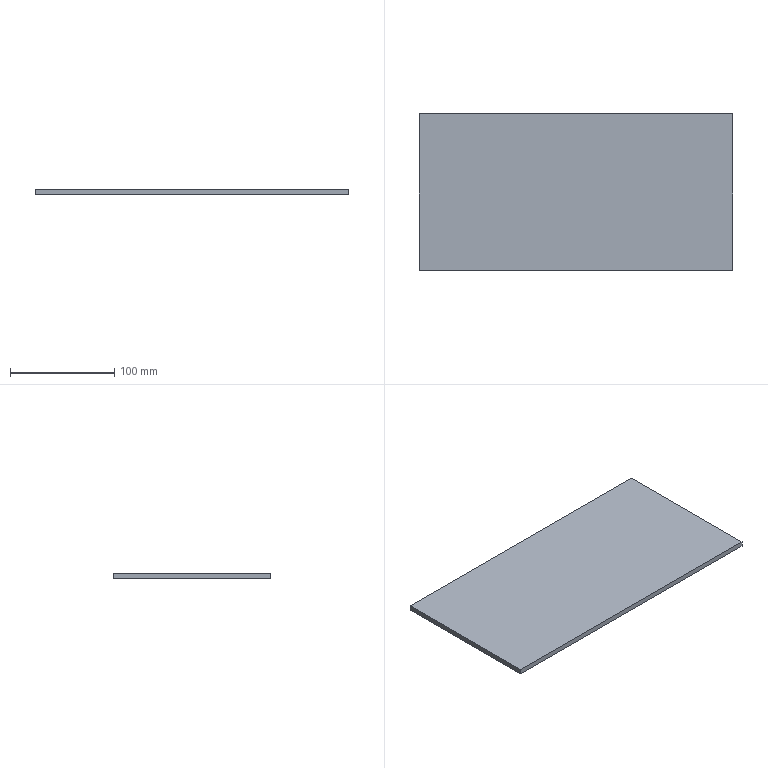Part | SolidWorks | features Extrusion 1 | 1 solid | 6 faces | box 300 x 150 x 5 mm | volume 225000 mm3 | plane 6
STEP:
#1=CARTESIAN_POINT('',(0.,150.,0.));
#2=VERTEX_POINT('',#1);
#3=CARTESIAN_POINT('',(0.,0.,0.));
#4=VERTEX_POINT('',#3);
#5=CARTESIAN_POINT('',(0.,0.,0.));
#6=DIRECTION('',(0.,-1.,0.));
#7=VECTOR('',#6,1000.);
#8=LINE('',#5,#7);
#9=EDGE_CURVE('',#2,#4,#8,.T.);
#10=ORIENTED_EDGE('',*,*,#9,.T.);
#11=CARTESIAN_POINT('',(0.,0.,5.));
#12=VERTEX_POINT('',#11);
#13=CARTESIAN_POINT('',(0.,0.,5.));
#14=DIRECTION('',(0.,0.,-1.));
#15=VECTOR('',#14,1000.);
#16=LINE('',#13,#15);
#17=EDGE_CURVE('',#12,#4,#16,.T.);
#18=ORIENTED_EDGE('',*,*,#17,.F.);
#19=CARTESIAN_POINT('',(0.,150.,5.));
#20=VERTEX_POINT('',#19);
#21=CARTESIAN_POINT('',(0.,0.,5.));
#22=DIRECTION('',(0.,-1.,0.));
#23=VECTOR('',#22,1000.);
#24=LINE('',#21,#23);
#25=EDGE_CURVE('',#20,#12,#24,.T.);
#26=ORIENTED_EDGE('',*,*,#25,.F.);
#27=CARTESIAN_POINT('',(0.,150.,5.));
#28=DIRECTION('',(0.,0.,-1.));
#29=VECTOR('',#28,1000.);
#30=LINE('',#27,#29);
#31=EDGE_CURVE('',#20,#2,#30,.T.);
#32=ORIENTED_EDGE('',*,*,#31,.T.);
#33=EDGE_LOOP('',(#10,#18,#26,#32));
#34=FACE_OUTER_BOUND('',#33,.T.);
#35=CARTESIAN_POINT('',(0.,0.,5.));
#36=DIRECTION('',(1.,0.,0.));
#37=DIRECTION('',(0.,0.,-1.));
#38=AXIS2_PLACEMENT_3D('',#35,#36,#37);
#39=PLANE('',#38);
#40=ADVANCED_FACE('',(#34),#39,.F.);
#41=CARTESIAN_POINT('',(300.,0.,0.));
#42=VERTEX_POINT('',#41);
#43=CARTESIAN_POINT('',(0.,0.,0.));
#44=DIRECTION('',(1.,0.,0.));
#45=VECTOR('',#44,1000.);
#46=LINE('',#43,#45);
#47=EDGE_CURVE('',#4,#42,#46,.T.);
#48=ORIENTED_EDGE('',*,*,#47,.T.);
#49=CARTESIAN_POINT('',(300.,0.,5.));
#50=VERTEX_POINT('',#49);
#51=CARTESIAN_POINT('',(300.,0.,5.));
#52=DIRECTION('',(0.,0.,-1.));
#53=VECTOR('',#52,1000.);
#54=LINE('',#51,#53);
#55=EDGE_CURVE('',#50,#42,#54,.T.);
#56=ORIENTED_EDGE('',*,*,#55,.F.);
#57=CARTESIAN_POINT('',(0.,0.,5.));
#58=DIRECTION('',(1.,0.,0.));
#59=VECTOR('',#58,1000.);
#60=LINE('',#57,#59);
#61=EDGE_CURVE('',#12,#50,#60,.T.);
#62=ORIENTED_EDGE('',*,*,#61,.F.);
#63=ORIENTED_EDGE('',*,*,#17,.T.);
#64=EDGE_LOOP('',(#48,#56,#62,#63));
#65=FACE_OUTER_BOUND('',#64,.T.);
#66=CARTESIAN_POINT('',(0.,0.,5.));
#67=DIRECTION('',(0.,1.,0.));
#68=DIRECTION('',(0.,0.,1.));
#69=AXIS2_PLACEMENT_3D('',#66,#67,#68);
#70=PLANE('',#69);
#71=ADVANCED_FACE('',(#65),#70,.F.);
#72=CARTESIAN_POINT('',(300.,150.,0.));
#73=VERTEX_POINT('',#72);
#74=CARTESIAN_POINT('',(300.,0.,0.));
#75=DIRECTION('',(0.,1.,0.));
#76=VECTOR('',#75,1000.);
#77=LINE('',#74,#76);
#78=EDGE_CURVE('',#42,#73,#77,.T.);
#79=ORIENTED_EDGE('',*,*,#78,.T.);
#80=CARTESIAN_POINT('',(300.,150.,5.));
#81=VERTEX_POINT('',#80);
#82=CARTESIAN_POINT('',(300.,150.,5.));
#83=DIRECTION('',(0.,0.,-1.));
#84=VECTOR('',#83,1000.);
#85=LINE('',#82,#84);
#86=EDGE_CURVE('',#81,#73,#85,.T.);
#87=ORIENTED_EDGE('',*,*,#86,.F.);
#88=CARTESIAN_POINT('',(300.,0.,5.));
#89=DIRECTION('',(0.,1.,0.));
#90=VECTOR('',#89,1000.);
#91=LINE('',#88,#90);
#92=EDGE_CURVE('',#50,#81,#91,.T.);
#93=ORIENTED_EDGE('',*,*,#92,.F.);
#94=ORIENTED_EDGE('',*,*,#55,.T.);
#95=EDGE_LOOP('',(#79,#87,#93,#94));
#96=FACE_OUTER_BOUND('',#95,.T.);
#97=CARTESIAN_POINT('',(300.,0.,5.));
#98=DIRECTION('',(-1.,0.,0.));
#99=DIRECTION('',(0.,0.,1.));
#100=AXIS2_PLACEMENT_3D('',#97,#98,#99);
#101=PLANE('',#100);
#102=ADVANCED_FACE('',(#96),#101,.F.);
#103=CARTESIAN_POINT('',(0.,150.,0.));
#104=DIRECTION('',(-1.,0.,0.));
#105=VECTOR('',#104,1000.);
#106=LINE('',#103,#105);
#107=EDGE_CURVE('',#73,#2,#106,.T.);
#108=ORIENTED_EDGE('',*,*,#107,.T.);
#109=ORIENTED_EDGE('',*,*,#31,.F.);
#110=CARTESIAN_POINT('',(0.,150.,5.));
#111=DIRECTION('',(-1.,0.,0.));
#112=VECTOR('',#111,1000.);
#113=LINE('',#110,#112);
#114=EDGE_CURVE('',#81,#20,#113,.T.);
#115=ORIENTED_EDGE('',*,*,#114,.F.);
#116=ORIENTED_EDGE('',*,*,#86,.T.);
#117=EDGE_LOOP('',(#108,#109,#115,#116));
#118=FACE_OUTER_BOUND('',#117,.T.);
#119=CARTESIAN_POINT('',(0.,150.,5.));
#120=DIRECTION('',(0.,-1.,0.));
#121=DIRECTION('',(0.,0.,-1.));
#122=AXIS2_PLACEMENT_3D('',#119,#120,#121);
#123=PLANE('',#122);
#124=ADVANCED_FACE('',(#118),#123,.F.);
#125=ORIENTED_EDGE('',*,*,#25,.T.);
#126=ORIENTED_EDGE('',*,*,#61,.T.);
#127=ORIENTED_EDGE('',*,*,#92,.T.);
#128=ORIENTED_EDGE('',*,*,#114,.T.);
#129=EDGE_LOOP('',(#125,#126,#127,#128));
#130=FACE_OUTER_BOUND('',#129,.T.);
#131=CARTESIAN_POINT('',(0.,0.,5.));
#132=DIRECTION('',(0.,0.,-1.));
#133=DIRECTION('',(-1.,0.,0.));
#134=AXIS2_PLACEMENT_3D('',#131,#132,#133);
#135=PLANE('',#134);
#136=ADVANCED_FACE('',(#130),#135,.F.);
#137=ORIENTED_EDGE('',*,*,#9,.F.);
#138=ORIENTED_EDGE('',*,*,#107,.F.);
#139=ORIENTED_EDGE('',*,*,#78,.F.);
#140=ORIENTED_EDGE('',*,*,#47,.F.);
#141=EDGE_LOOP('',(#137,#138,#139,#140));
#142=FACE_OUTER_BOUND('',#141,.T.);
#143=CARTESIAN_POINT('',(0.,0.,0.));
#144=DIRECTION('',(0.,0.,-1.));
#145=DIRECTION('',(-1.,0.,0.));
#146=AXIS2_PLACEMENT_3D('',#143,#144,#145);
#147=PLANE('',#146);
#148=ADVANCED_FACE('',(#142),#147,.T.);
#149=CLOSED_SHELL('',(#40,#71,#102,#124,#136,#148));
#150=MANIFOLD_SOLID_BREP('',#149);
#151=CARTESIAN_POINT('',(0.,0.,0.));
#152=DIRECTION('',(0.,0.,1.));
#153=DIRECTION('',(1.,0.,0.));
#154=AXIS2_PLACEMENT_3D('',#151,#152,#153);
#155=(LENGTH_UNIT()NAMED_UNIT(*)SI_UNIT(.MILLI.,.METRE.));
#156=UNCERTAINTY_MEASURE_WITH_UNIT(LENGTH_MEASURE(0.00001),#155,'','');
#157=(NAMED_UNIT(*)PLANE_ANGLE_UNIT()SI_UNIT($,.RADIAN.));
#158=(NAMED_UNIT(*)SI_UNIT($,.STERADIAN.)SOLID_ANGLE_UNIT());
#159=(GEOMETRIC_REPRESENTATION_CONTEXT(3)GLOBAL_UNCERTAINTY_ASSIGNED_CONTEXT((#156))GLOBAL_UNIT_ASSIGNED_CONTEXT((#155,#157,#158))REPRESENTATION_CONTEXT('',''));
#160=ADVANCED_BREP_SHAPE_REPRESENTATION('',(#150,#154),#159);